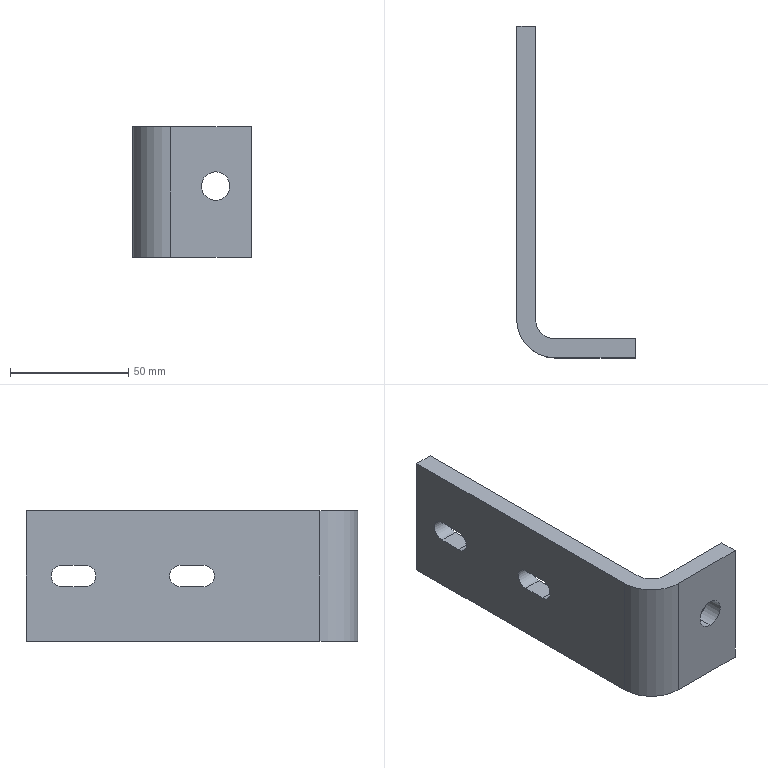Part | STEP file | X77-03031 | 1 solid | 20 faces | box 50 x 140 x 55 mm | volume 74451 mm3 | plane 12 | cylinder 8 | commonest cylinder face diameters 9 x4 12 x2 16 x1 32 x1
STEP:
#1=CARTESIAN_POINT('',(-687.13,-4694.875,24.));
#2=VERTEX_POINT('',#1);
#3=CARTESIAN_POINT('',(-687.13,-4694.875,36.));
#4=VERTEX_POINT('',#3);
#5=CARTESIAN_POINT('',(-687.13,-4694.875,30.));
#6=DIRECTION('',(0.,1.,0.));
#7=DIRECTION('',(0.,0.,1.));
#8=AXIS2_PLACEMENT_3D('',#5,#6,#7);
#9=CIRCLE('',#8,6.);
#10=EDGE_CURVE('',#2,#4,#9,.T.);
#11=ORIENTED_EDGE('',*,*,#10,.F.);
#12=CARTESIAN_POINT('',(-687.13,-4686.875,24.));
#13=VERTEX_POINT('',#12);
#14=CARTESIAN_POINT('',(-687.13,-4746.875,24.));
#15=DIRECTION('',(0.,1.,0.));
#16=VECTOR('',#15,1000.);
#17=LINE('',#14,#16);
#18=EDGE_CURVE('',#2,#13,#17,.T.);
#19=ORIENTED_EDGE('',*,*,#18,.T.);
#20=CARTESIAN_POINT('',(-687.13,-4686.875,36.));
#21=VERTEX_POINT('',#20);
#22=CARTESIAN_POINT('',(-687.13,-4686.875,30.));
#23=DIRECTION('',(0.,1.,0.));
#24=DIRECTION('',(0.,0.,1.));
#25=AXIS2_PLACEMENT_3D('',#22,#23,#24);
#26=CIRCLE('',#25,6.);
#27=EDGE_CURVE('',#13,#21,#26,.T.);
#28=ORIENTED_EDGE('',*,*,#27,.T.);
#29=CARTESIAN_POINT('',(-687.13,-4746.875,36.));
#30=DIRECTION('',(0.,1.,0.));
#31=VECTOR('',#30,1000.);
#32=LINE('',#29,#31);
#33=EDGE_CURVE('',#4,#21,#32,.T.);
#34=ORIENTED_EDGE('',*,*,#33,.F.);
#35=EDGE_LOOP('',(#11,#19,#28,#34));
#36=FACE_OUTER_BOUND('',#35,.T.);
#37=CARTESIAN_POINT('',(-687.13,-4746.875,30.));
#38=DIRECTION('',(0.,1.,0.));
#39=DIRECTION('',(0.,0.,1.));
#40=AXIS2_PLACEMENT_3D('',#37,#38,#39);
#41=CYLINDRICAL_SURFACE('',#40,6.);
#42=ADVANCED_FACE('',(#36),#41,.F.);
#43=CARTESIAN_POINT('',(-714.13,-4554.875,0.));
#44=VERTEX_POINT('',#43);
#45=CARTESIAN_POINT('',(-722.13,-4554.875,0.));
#46=VERTEX_POINT('',#45);
#47=CARTESIAN_POINT('',(-722.13,-4554.875,0.));
#48=DIRECTION('',(-1.,0.,0.));
#49=VECTOR('',#48,1000.);
#50=LINE('',#47,#49);
#51=EDGE_CURVE('',#44,#46,#50,.T.);
#52=ORIENTED_EDGE('',*,*,#51,.T.);
#53=CARTESIAN_POINT('',(-722.13,-4554.875,55.));
#54=VERTEX_POINT('',#53);
#55=CARTESIAN_POINT('',(-722.13,-4554.875,55.));
#56=DIRECTION('',(0.,0.,-1.));
#57=VECTOR('',#56,1000.);
#58=LINE('',#55,#57);
#59=EDGE_CURVE('',#54,#46,#58,.T.);
#60=ORIENTED_EDGE('',*,*,#59,.F.);
#61=CARTESIAN_POINT('',(-714.13,-4554.875,55.));
#62=VERTEX_POINT('',#61);
#63=CARTESIAN_POINT('',(-722.13,-4554.875,55.));
#64=DIRECTION('',(-1.,0.,0.));
#65=VECTOR('',#64,1000.);
#66=LINE('',#63,#65);
#67=EDGE_CURVE('',#62,#54,#66,.T.);
#68=ORIENTED_EDGE('',*,*,#67,.F.);
#69=CARTESIAN_POINT('',(-714.13,-4554.875,55.));
#70=DIRECTION('',(0.,0.,-1.));
#71=VECTOR('',#70,1000.);
#72=LINE('',#69,#71);
#73=EDGE_CURVE('',#62,#44,#72,.T.);
#74=ORIENTED_EDGE('',*,*,#73,.T.);
#75=EDGE_LOOP('',(#52,#60,#68,#74));
#76=FACE_OUTER_BOUND('',#75,.T.);
#77=CARTESIAN_POINT('',(-722.13,-4554.875,55.));
#78=DIRECTION('',(0.,-1.,0.));
#79=DIRECTION('',(0.,0.,-1.));
#80=AXIS2_PLACEMENT_3D('',#77,#78,#79);
#81=PLANE('',#80);
#82=ADVANCED_FACE('',(#76),#81,.F.);
#83=CARTESIAN_POINT('',(-722.13,-4619.875,32.));
#84=VERTEX_POINT('',#83);
#85=CARTESIAN_POINT('',(-722.13,-4629.875,32.));
#86=VERTEX_POINT('',#85);
#87=CARTESIAN_POINT('',(-722.13,-4554.875,32.));
#88=DIRECTION('',(0.,-1.,0.));
#89=VECTOR('',#88,1000.);
#90=LINE('',#87,#89);
#91=EDGE_CURVE('',#84,#86,#90,.T.);
#92=ORIENTED_EDGE('',*,*,#91,.T.);
#93=CARTESIAN_POINT('',(-722.13,-4629.875,23.));
#94=VERTEX_POINT('',#93);
#95=CARTESIAN_POINT('',(-722.13,-4629.875,27.5));
#96=DIRECTION('',(1.,0.,0.));
#97=DIRECTION('',(0.,0.,-1.));
#98=AXIS2_PLACEMENT_3D('',#95,#96,#97);
#99=CIRCLE('',#98,4.5);
#100=EDGE_CURVE('',#86,#94,#99,.T.);
#101=ORIENTED_EDGE('',*,*,#100,.T.);
#102=CARTESIAN_POINT('',(-722.13,-4619.875,23.));
#103=VERTEX_POINT('',#102);
#104=CARTESIAN_POINT('',(-722.13,-4554.875,23.));
#105=DIRECTION('',(0.,1.,0.));
#106=VECTOR('',#105,1000.);
#107=LINE('',#104,#106);
#108=EDGE_CURVE('',#94,#103,#107,.T.);
#109=ORIENTED_EDGE('',*,*,#108,.T.);
#110=CARTESIAN_POINT('',(-722.13,-4619.875,27.5));
#111=DIRECTION('',(1.,0.,0.));
#112=DIRECTION('',(0.,0.,-1.));
#113=AXIS2_PLACEMENT_3D('',#110,#111,#112);
#114=CIRCLE('',#113,4.5);
#115=EDGE_CURVE('',#103,#84,#114,.T.);
#116=ORIENTED_EDGE('',*,*,#115,.T.);
#117=EDGE_LOOP('',(#92,#101,#109,#116));
#118=FACE_BOUND('',#117,.T.);
#119=CARTESIAN_POINT('',(-722.13,-4579.875,23.));
#120=VERTEX_POINT('',#119);
#121=CARTESIAN_POINT('',(-722.13,-4569.875,23.));
#122=VERTEX_POINT('',#121);
#123=CARTESIAN_POINT('',(-722.13,-4554.875,23.));
#124=DIRECTION('',(0.,1.,0.));
#125=VECTOR('',#124,1000.);
#126=LINE('',#123,#125);
#127=EDGE_CURVE('',#120,#122,#126,.T.);
#128=ORIENTED_EDGE('',*,*,#127,.T.);
#129=CARTESIAN_POINT('',(-722.13,-4569.875,32.));
#130=VERTEX_POINT('',#129);
#131=CARTESIAN_POINT('',(-722.13,-4569.875,27.5));
#132=DIRECTION('',(1.,0.,0.));
#133=DIRECTION('',(0.,0.,-1.));
#134=AXIS2_PLACEMENT_3D('',#131,#132,#133);
#135=CIRCLE('',#134,4.5);
#136=EDGE_CURVE('',#122,#130,#135,.T.);
#137=ORIENTED_EDGE('',*,*,#136,.T.);
#138=CARTESIAN_POINT('',(-722.13,-4579.875,32.));
#139=VERTEX_POINT('',#138);
#140=CARTESIAN_POINT('',(-722.13,-4554.875,32.));
#141=DIRECTION('',(0.,-1.,0.));
#142=VECTOR('',#141,1000.);
#143=LINE('',#140,#142);
#144=EDGE_CURVE('',#130,#139,#143,.T.);
#145=ORIENTED_EDGE('',*,*,#144,.T.);
#146=CARTESIAN_POINT('',(-722.13,-4579.875,27.5));
#147=DIRECTION('',(1.,0.,0.));
#148=DIRECTION('',(0.,0.,-1.));
#149=AXIS2_PLACEMENT_3D('',#146,#147,#148);
#150=CIRCLE('',#149,4.5);
#151=EDGE_CURVE('',#139,#120,#150,.T.);
#152=ORIENTED_EDGE('',*,*,#151,.T.);
#153=EDGE_LOOP('',(#128,#137,#145,#152));
#154=FACE_BOUND('',#153,.T.);
#155=CARTESIAN_POINT('',(-722.13,-4678.875,0.));
#156=VERTEX_POINT('',#155);
#157=CARTESIAN_POINT('',(-722.13,-4554.875,0.));
#158=DIRECTION('',(0.,-1.,0.));
#159=VECTOR('',#158,1000.);
#160=LINE('',#157,#159);
#161=EDGE_CURVE('',#46,#156,#160,.T.);
#162=ORIENTED_EDGE('',*,*,#161,.T.);
#163=CARTESIAN_POINT('',(-722.13,-4678.875,55.));
#164=VERTEX_POINT('',#163);
#165=CARTESIAN_POINT('',(-722.13,-4678.875,55.));
#166=DIRECTION('',(0.,0.,1.));
#167=VECTOR('',#166,1000.);
#168=LINE('',#165,#167);
#169=EDGE_CURVE('',#156,#164,#168,.T.);
#170=ORIENTED_EDGE('',*,*,#169,.T.);
#171=CARTESIAN_POINT('',(-722.13,-4554.875,55.));
#172=DIRECTION('',(0.,-1.,0.));
#173=VECTOR('',#172,1000.);
#174=LINE('',#171,#173);
#175=EDGE_CURVE('',#54,#164,#174,.T.);
#176=ORIENTED_EDGE('',*,*,#175,.F.);
#177=ORIENTED_EDGE('',*,*,#59,.T.);
#178=EDGE_LOOP('',(#162,#170,#176,#177));
#179=FACE_OUTER_BOUND('',#178,.T.);
#180=CARTESIAN_POINT('',(-722.13,-4554.875,55.));
#181=DIRECTION('',(1.,0.,0.));
#182=DIRECTION('',(0.,0.,-1.));
#183=AXIS2_PLACEMENT_3D('',#180,#181,#182);
#184=PLANE('',#183);
#185=ADVANCED_FACE('',(#118,#154,#179),#184,.F.);
#186=CARTESIAN_POINT('',(-687.13,-4694.875,30.));
#187=DIRECTION('',(0.,1.,0.));
#188=DIRECTION('',(0.,0.,1.));
#189=AXIS2_PLACEMENT_3D('',#186,#187,#188);
#190=CIRCLE('',#189,6.);
#191=EDGE_CURVE('',#4,#2,#190,.T.);
#192=ORIENTED_EDGE('',*,*,#191,.T.);
#193=ORIENTED_EDGE('',*,*,#10,.T.);
#194=EDGE_LOOP('',(#192,#193));
#195=FACE_BOUND('',#194,.T.);
#196=CARTESIAN_POINT('',(-706.13,-4694.875,55.));
#197=VERTEX_POINT('',#196);
#198=CARTESIAN_POINT('',(-672.13,-4694.875,55.));
#199=VERTEX_POINT('',#198);
#200=CARTESIAN_POINT('',(-672.13,-4694.875,55.));
#201=DIRECTION('',(1.,0.,0.));
#202=VECTOR('',#201,1000.);
#203=LINE('',#200,#202);
#204=EDGE_CURVE('',#197,#199,#203,.T.);
#205=ORIENTED_EDGE('',*,*,#204,.F.);
#206=CARTESIAN_POINT('',(-706.13,-4694.875,0.));
#207=VERTEX_POINT('',#206);
#208=CARTESIAN_POINT('',(-706.13,-4694.875,55.));
#209=DIRECTION('',(0.,0.,-1.));
#210=VECTOR('',#209,1000.);
#211=LINE('',#208,#210);
#212=EDGE_CURVE('',#197,#207,#211,.T.);
#213=ORIENTED_EDGE('',*,*,#212,.T.);
#214=CARTESIAN_POINT('',(-672.13,-4694.875,0.));
#215=VERTEX_POINT('',#214);
#216=CARTESIAN_POINT('',(-672.13,-4694.875,0.));
#217=DIRECTION('',(1.,0.,0.));
#218=VECTOR('',#217,1000.);
#219=LINE('',#216,#218);
#220=EDGE_CURVE('',#207,#215,#219,.T.);
#221=ORIENTED_EDGE('',*,*,#220,.T.);
#222=CARTESIAN_POINT('',(-672.13,-4694.875,55.));
#223=DIRECTION('',(0.,0.,-1.));
#224=VECTOR('',#223,1000.);
#225=LINE('',#222,#224);
#226=EDGE_CURVE('',#199,#215,#225,.T.);
#227=ORIENTED_EDGE('',*,*,#226,.F.);
#228=EDGE_LOOP('',(#205,#213,#221,#227));
#229=FACE_OUTER_BOUND('',#228,.T.);
#230=CARTESIAN_POINT('',(-672.13,-4694.875,55.));
#231=DIRECTION('',(0.,1.,0.));
#232=DIRECTION('',(0.,0.,1.));
#233=AXIS2_PLACEMENT_3D('',#230,#231,#232);
#234=PLANE('',#233);
#235=ADVANCED_FACE('',(#195,#229),#234,.F.);
#236=CARTESIAN_POINT('',(-672.13,-4686.875,0.));
#237=VERTEX_POINT('',#236);
#238=CARTESIAN_POINT('',(-672.13,-4686.875,0.));
#239=DIRECTION('',(0.,1.,0.));
#240=VECTOR('',#239,1000.);
#241=LINE('',#238,#240);
#242=EDGE_CURVE('',#215,#237,#241,.T.);
#243=ORIENTED_EDGE('',*,*,#242,.T.);
#244=CARTESIAN_POINT('',(-672.13,-4686.875,55.));
#245=VERTEX_POINT('',#244);
#246=CARTESIAN_POINT('',(-672.13,-4686.875,55.));
#247=DIRECTION('',(0.,0.,-1.));
#248=VECTOR('',#247,1000.);
#249=LINE('',#246,#248);
#250=EDGE_CURVE('',#245,#237,#249,.T.);
#251=ORIENTED_EDGE('',*,*,#250,.F.);
#252=CARTESIAN_POINT('',(-672.13,-4686.875,55.));
#253=DIRECTION('',(0.,1.,0.));
#254=VECTOR('',#253,1000.);
#255=LINE('',#252,#254);
#256=EDGE_CURVE('',#199,#245,#255,.T.);
#257=ORIENTED_EDGE('',*,*,#256,.F.);
#258=ORIENTED_EDGE('',*,*,#226,.T.);
#259=EDGE_LOOP('',(#243,#251,#257,#258));
#260=FACE_OUTER_BOUND('',#259,.T.);
#261=CARTESIAN_POINT('',(-672.13,-4686.875,55.));
#262=DIRECTION('',(-1.,0.,0.));
#263=DIRECTION('',(0.,0.,1.));
#264=AXIS2_PLACEMENT_3D('',#261,#262,#263);
#265=PLANE('',#264);
#266=ADVANCED_FACE('',(#260),#265,.F.);
#267=CARTESIAN_POINT('',(-687.13,-4686.875,30.));
#268=DIRECTION('',(0.,1.,0.));
#269=DIRECTION('',(0.,0.,1.));
#270=AXIS2_PLACEMENT_3D('',#267,#268,#269);
#271=CIRCLE('',#270,6.);
#272=EDGE_CURVE('',#21,#13,#271,.T.);
#273=ORIENTED_EDGE('',*,*,#272,.F.);
#274=ORIENTED_EDGE('',*,*,#27,.F.);
#275=EDGE_LOOP('',(#273,#274));
#276=FACE_BOUND('',#275,.T.);
#277=CARTESIAN_POINT('',(-706.13,-4686.875,0.));
#278=VERTEX_POINT('',#277);
#279=CARTESIAN_POINT('',(-714.13,-4686.875,0.));
#280=DIRECTION('',(-1.,0.,0.));
#281=VECTOR('',#280,1000.);
#282=LINE('',#279,#281);
#283=EDGE_CURVE('',#237,#278,#282,.T.);
#284=ORIENTED_EDGE('',*,*,#283,.T.);
#285=CARTESIAN_POINT('',(-706.13,-4686.875,55.));
#286=VERTEX_POINT('',#285);
#287=CARTESIAN_POINT('',(-706.13,-4686.875,55.));
#288=DIRECTION('',(0.,0.,1.));
#289=VECTOR('',#288,1000.);
#290=LINE('',#287,#289);
#291=EDGE_CURVE('',#278,#286,#290,.T.);
#292=ORIENTED_EDGE('',*,*,#291,.T.);
#293=CARTESIAN_POINT('',(-714.13,-4686.875,55.));
#294=DIRECTION('',(-1.,0.,0.));
#295=VECTOR('',#294,1000.);
#296=LINE('',#293,#295);
#297=EDGE_CURVE('',#245,#286,#296,.T.);
#298=ORIENTED_EDGE('',*,*,#297,.F.);
#299=ORIENTED_EDGE('',*,*,#250,.T.);
#300=EDGE_LOOP('',(#284,#292,#298,#299));
#301=FACE_OUTER_BOUND('',#300,.T.);
#302=CARTESIAN_POINT('',(-714.13,-4686.875,55.));
#303=DIRECTION('',(0.,-1.,0.));
#304=DIRECTION('',(0.,0.,-1.));
#305=AXIS2_PLACEMENT_3D('',#302,#303,#304);
#306=PLANE('',#305);
#307=ADVANCED_FACE('',(#276,#301),#306,.F.);
#308=CARTESIAN_POINT('',(-714.13,-4629.875,23.));
#309=VERTEX_POINT('',#308);
#310=CARTESIAN_POINT('',(-714.13,-4619.875,23.));
#311=VERTEX_POINT('',#310);
#312=CARTESIAN_POINT('',(-714.13,-4629.875,23.));
#313=DIRECTION('',(0.,1.,0.));
#314=VECTOR('',#313,1000.);
#315=LINE('',#312,#314);
#316=EDGE_CURVE('',#309,#311,#315,.T.);
#317=ORIENTED_EDGE('',*,*,#316,.F.);
#318=CARTESIAN_POINT('',(-714.13,-4629.875,32.));
#319=VERTEX_POINT('',#318);
#320=CARTESIAN_POINT('',(-714.13,-4629.875,27.5));
#321=DIRECTION('',(1.,0.,0.));
#322=DIRECTION('',(0.,0.,-1.));
#323=AXIS2_PLACEMENT_3D('',#320,#321,#322);
#324=CIRCLE('',#323,4.5);
#325=EDGE_CURVE('',#319,#309,#324,.T.);
#326=ORIENTED_EDGE('',*,*,#325,.F.);
#327=CARTESIAN_POINT('',(-714.13,-4619.875,32.));
#328=VERTEX_POINT('',#327);
#329=CARTESIAN_POINT('',(-714.13,-4629.875,32.));
#330=DIRECTION('',(0.,-1.,0.));
#331=VECTOR('',#330,1000.);
#332=LINE('',#329,#331);
#333=EDGE_CURVE('',#328,#319,#332,.T.);
#334=ORIENTED_EDGE('',*,*,#333,.F.);
#335=CARTESIAN_POINT('',(-714.13,-4619.875,27.5));
#336=DIRECTION('',(1.,0.,0.));
#337=DIRECTION('',(0.,0.,-1.));
#338=AXIS2_PLACEMENT_3D('',#335,#336,#337);
#339=CIRCLE('',#338,4.5);
#340=EDGE_CURVE('',#311,#328,#339,.T.);
#341=ORIENTED_EDGE('',*,*,#340,.F.);
#342=EDGE_LOOP('',(#317,#326,#334,#341));
#343=FACE_BOUND('',#342,.T.);
#344=CARTESIAN_POINT('',(-714.13,-4569.875,32.));
#345=VERTEX_POINT('',#344);
#346=CARTESIAN_POINT('',(-714.13,-4579.875,32.));
#347=VERTEX_POINT('',#346);
#348=CARTESIAN_POINT('',(-714.13,-4569.875,32.));
#349=DIRECTION('',(0.,-1.,0.));
#350=VECTOR('',#349,1000.);
#351=LINE('',#348,#350);
#352=EDGE_CURVE('',#345,#347,#351,.T.);
#353=ORIENTED_EDGE('',*,*,#352,.F.);
#354=CARTESIAN_POINT('',(-714.13,-4569.875,23.));
#355=VERTEX_POINT('',#354);
#356=CARTESIAN_POINT('',(-714.13,-4569.875,27.5));
#357=DIRECTION('',(1.,0.,0.));
#358=DIRECTION('',(0.,0.,-1.));
#359=AXIS2_PLACEMENT_3D('',#356,#357,#358);
#360=CIRCLE('',#359,4.5);
#361=EDGE_CURVE('',#355,#345,#360,.T.);
#362=ORIENTED_EDGE('',*,*,#361,.F.);
#363=CARTESIAN_POINT('',(-714.13,-4579.875,23.));
#364=VERTEX_POINT('',#363);
#365=CARTESIAN_POINT('',(-714.13,-4569.875,23.));
#366=DIRECTION('',(0.,1.,0.));
#367=VECTOR('',#366,1000.);
#368=LINE('',#365,#367);
#369=EDGE_CURVE('',#364,#355,#368,.T.);
#370=ORIENTED_EDGE('',*,*,#369,.F.);
#371=CARTESIAN_POINT('',(-714.13,-4579.875,27.5));
#372=DIRECTION('',(1.,0.,0.));
#373=DIRECTION('',(0.,0.,-1.));
#374=AXIS2_PLACEMENT_3D('',#371,#372,#373);
#375=CIRCLE('',#374,4.5);
#376=EDGE_CURVE('',#347,#364,#375,.T.);
#377=ORIENTED_EDGE('',*,*,#376,.F.);
#378=EDGE_LOOP('',(#353,#362,#370,#377));
#379=FACE_BOUND('',#378,.T.);
#380=CARTESIAN_POINT('',(-714.13,-4678.875,55.));
#381=VERTEX_POINT('',#380);
#382=CARTESIAN_POINT('',(-714.13,-4554.875,55.));
#383=DIRECTION('',(0.,1.,0.));
#384=VECTOR('',#383,1000.);
#385=LINE('',#382,#384);
#386=EDGE_CURVE('',#381,#62,#385,.T.);
#387=ORIENTED_EDGE('',*,*,#386,.F.);
#388=CARTESIAN_POINT('',(-714.13,-4678.875,0.));
#389=VERTEX_POINT('',#388);
#390=CARTESIAN_POINT('',(-714.13,-4678.875,0.));
#391=DIRECTION('',(0.,0.,-1.));
#392=VECTOR('',#391,1000.);
#393=LINE('',#390,#392);
#394=EDGE_CURVE('',#381,#389,#393,.T.);
#395=ORIENTED_EDGE('',*,*,#394,.T.);
#396=CARTESIAN_POINT('',(-714.13,-4554.875,0.));
#397=DIRECTION('',(0.,1.,0.));
#398=VECTOR('',#397,1000.);
#399=LINE('',#396,#398);
#400=EDGE_CURVE('',#389,#44,#399,.T.);
#401=ORIENTED_EDGE('',*,*,#400,.T.);
#402=ORIENTED_EDGE('',*,*,#73,.F.);
#403=EDGE_LOOP('',(#387,#395,#401,#402));
#404=FACE_OUTER_BOUND('',#403,.T.);
#405=CARTESIAN_POINT('',(-714.13,-4554.875,55.));
#406=DIRECTION('',(-1.,0.,0.));
#407=DIRECTION('',(0.,0.,1.));
#408=AXIS2_PLACEMENT_3D('',#405,#406,#407);
#409=PLANE('',#408);
#410=ADVANCED_FACE('',(#343,#379,#404),#409,.F.);
#411=ORIENTED_EDGE('',*,*,#175,.T.);
#412=CARTESIAN_POINT('',(-706.13,-4678.875,55.));
#413=DIRECTION('',(0.,0.,1.));
#414=DIRECTION('',(-1.,0.,0.));
#415=AXIS2_PLACEMENT_3D('',#412,#413,#414);
#416=CIRCLE('',#415,16.);
#417=EDGE_CURVE('',#164,#197,#416,.T.);
#418=ORIENTED_EDGE('',*,*,#417,.T.);
#419=ORIENTED_EDGE('',*,*,#204,.T.);
#420=ORIENTED_EDGE('',*,*,#256,.T.);
#421=ORIENTED_EDGE('',*,*,#297,.T.);
#422=CARTESIAN_POINT('',(-706.13,-4678.875,55.));
#423=DIRECTION('',(0.,0.,-1.));
#424=DIRECTION('',(-1.,0.,0.));
#425=AXIS2_PLACEMENT_3D('',#422,#423,#424);
#426=CIRCLE('',#425,8.);
#427=EDGE_CURVE('',#286,#381,#426,.T.);
#428=ORIENTED_EDGE('',*,*,#427,.T.);
#429=ORIENTED_EDGE('',*,*,#386,.T.);
#430=ORIENTED_EDGE('',*,*,#67,.T.);
#431=EDGE_LOOP('',(#411,#418,#419,#420,#421,#428,#429,#430));
#432=FACE_OUTER_BOUND('',#431,.T.);
#433=CARTESIAN_POINT('',(-714.13,-4554.875,55.));
#434=DIRECTION('',(0.,0.,-1.));
#435=DIRECTION('',(-1.,0.,0.));
#436=AXIS2_PLACEMENT_3D('',#433,#434,#435);
#437=PLANE('',#436);
#438=ADVANCED_FACE('',(#432),#437,.F.);
#439=ORIENTED_EDGE('',*,*,#220,.F.);
#440=CARTESIAN_POINT('',(-706.13,-4678.875,0.));
#441=DIRECTION('',(0.,0.,-1.));
#442=DIRECTION('',(-1.,0.,0.));
#443=AXIS2_PLACEMENT_3D('',#440,#441,#442);
#444=CIRCLE('',#443,16.);
#445=EDGE_CURVE('',#207,#156,#444,.T.);
#446=ORIENTED_EDGE('',*,*,#445,.T.);
#447=ORIENTED_EDGE('',*,*,#161,.F.);
#448=ORIENTED_EDGE('',*,*,#51,.F.);
#449=ORIENTED_EDGE('',*,*,#400,.F.);
#450=CARTESIAN_POINT('',(-706.13,-4678.875,0.));
#451=DIRECTION('',(0.,0.,1.));
#452=DIRECTION('',(-1.,0.,0.));
#453=AXIS2_PLACEMENT_3D('',#450,#451,#452);
#454=CIRCLE('',#453,8.);
#455=EDGE_CURVE('',#389,#278,#454,.T.);
#456=ORIENTED_EDGE('',*,*,#455,.T.);
#457=ORIENTED_EDGE('',*,*,#283,.F.);
#458=ORIENTED_EDGE('',*,*,#242,.F.);
#459=EDGE_LOOP('',(#439,#446,#447,#448,#449,#456,#457,#458));
#460=FACE_OUTER_BOUND('',#459,.T.);
#461=CARTESIAN_POINT('',(-714.13,-4554.875,0.));
#462=DIRECTION('',(0.,0.,-1.));
#463=DIRECTION('',(-1.,0.,0.));
#464=AXIS2_PLACEMENT_3D('',#461,#462,#463);
#465=PLANE('',#464);
#466=ADVANCED_FACE('',(#460),#465,.T.);
#467=ORIENTED_EDGE('',*,*,#18,.F.);
#468=ORIENTED_EDGE('',*,*,#191,.F.);
#469=ORIENTED_EDGE('',*,*,#33,.T.);
#470=ORIENTED_EDGE('',*,*,#272,.T.);
#471=EDGE_LOOP('',(#467,#468,#469,#470));
#472=FACE_OUTER_BOUND('',#471,.T.);
#473=CARTESIAN_POINT('',(-687.13,-4746.875,30.));
#474=DIRECTION('',(0.,1.,0.));
#475=DIRECTION('',(0.,0.,1.));
#476=AXIS2_PLACEMENT_3D('',#473,#474,#475);
#477=CYLINDRICAL_SURFACE('',#476,6.);
#478=ADVANCED_FACE('',(#472),#477,.F.);
#479=ORIENTED_EDGE('',*,*,#427,.F.);
#480=ORIENTED_EDGE('',*,*,#291,.F.);
#481=ORIENTED_EDGE('',*,*,#455,.F.);
#482=ORIENTED_EDGE('',*,*,#394,.F.);
#483=EDGE_LOOP('',(#479,#480,#481,#482));
#484=FACE_OUTER_BOUND('',#483,.T.);
#485=CARTESIAN_POINT('',(-706.13,-4678.875,55.));
#486=DIRECTION('',(0.,0.,1.));
#487=DIRECTION('',(1.,0.,0.));
#488=AXIS2_PLACEMENT_3D('',#485,#486,#487);
#489=CYLINDRICAL_SURFACE('',#488,8.);
#490=ADVANCED_FACE('',(#484),#489,.F.);
#491=ORIENTED_EDGE('',*,*,#417,.F.);
#492=ORIENTED_EDGE('',*,*,#169,.F.);
#493=ORIENTED_EDGE('',*,*,#445,.F.);
#494=ORIENTED_EDGE('',*,*,#212,.F.);
#495=EDGE_LOOP('',(#491,#492,#493,#494));
#496=FACE_OUTER_BOUND('',#495,.T.);
#497=CARTESIAN_POINT('',(-706.13,-4678.875,55.));
#498=DIRECTION('',(0.,0.,-1.));
#499=DIRECTION('',(-1.,0.,0.));
#500=AXIS2_PLACEMENT_3D('',#497,#498,#499);
#501=CYLINDRICAL_SURFACE('',#500,16.);
#502=ADVANCED_FACE('',(#496),#501,.T.);
#503=CARTESIAN_POINT('',(-774.13,-4569.875,23.));
#504=DIRECTION('',(1.,0.,0.));
#505=VECTOR('',#504,1000.);
#506=LINE('',#503,#505);
#507=EDGE_CURVE('',#122,#355,#506,.T.);
#508=ORIENTED_EDGE('',*,*,#507,.T.);
#509=ORIENTED_EDGE('',*,*,#361,.T.);
#510=CARTESIAN_POINT('',(-774.13,-4569.875,32.));
#511=DIRECTION('',(1.,0.,0.));
#512=VECTOR('',#511,1000.);
#513=LINE('',#510,#512);
#514=EDGE_CURVE('',#130,#345,#513,.T.);
#515=ORIENTED_EDGE('',*,*,#514,.F.);
#516=ORIENTED_EDGE('',*,*,#136,.F.);
#517=EDGE_LOOP('',(#508,#509,#515,#516));
#518=FACE_OUTER_BOUND('',#517,.T.);
#519=CARTESIAN_POINT('',(-774.13,-4569.875,27.5));
#520=DIRECTION('',(1.,0.,0.));
#521=DIRECTION('',(0.,0.,-1.));
#522=AXIS2_PLACEMENT_3D('',#519,#520,#521);
#523=CYLINDRICAL_SURFACE('',#522,4.5);
#524=ADVANCED_FACE('',(#518),#523,.F.);
#525=CARTESIAN_POINT('',(-774.13,-4579.875,23.));
#526=DIRECTION('',(1.,0.,0.));
#527=VECTOR('',#526,1000.);
#528=LINE('',#525,#527);
#529=EDGE_CURVE('',#120,#364,#528,.T.);
#530=ORIENTED_EDGE('',*,*,#529,.T.);
#531=ORIENTED_EDGE('',*,*,#369,.T.);
#532=ORIENTED_EDGE('',*,*,#507,.F.);
#533=ORIENTED_EDGE('',*,*,#127,.F.);
#534=EDGE_LOOP('',(#530,#531,#532,#533));
#535=FACE_OUTER_BOUND('',#534,.T.);
#536=CARTESIAN_POINT('',(-774.13,-4569.875,23.));
#537=DIRECTION('',(0.,0.,-1.));
#538=DIRECTION('',(0.,1.,0.));
#539=AXIS2_PLACEMENT_3D('',#536,#537,#538);
#540=PLANE('',#539);
#541=ADVANCED_FACE('',(#535),#540,.F.);
#542=CARTESIAN_POINT('',(-774.13,-4579.875,32.));
#543=DIRECTION('',(1.,0.,0.));
#544=VECTOR('',#543,1000.);
#545=LINE('',#542,#544);
#546=EDGE_CURVE('',#139,#347,#545,.T.);
#547=ORIENTED_EDGE('',*,*,#546,.T.);
#548=ORIENTED_EDGE('',*,*,#376,.T.);
#549=ORIENTED_EDGE('',*,*,#529,.F.);
#550=ORIENTED_EDGE('',*,*,#151,.F.);
#551=EDGE_LOOP('',(#547,#548,#549,#550));
#552=FACE_OUTER_BOUND('',#551,.T.);
#553=CARTESIAN_POINT('',(-774.13,-4579.875,27.5));
#554=DIRECTION('',(1.,0.,0.));
#555=DIRECTION('',(0.,0.,-1.));
#556=AXIS2_PLACEMENT_3D('',#553,#554,#555);
#557=CYLINDRICAL_SURFACE('',#556,4.5);
#558=ADVANCED_FACE('',(#552),#557,.F.);
#559=ORIENTED_EDGE('',*,*,#514,.T.);
#560=ORIENTED_EDGE('',*,*,#352,.T.);
#561=ORIENTED_EDGE('',*,*,#546,.F.);
#562=ORIENTED_EDGE('',*,*,#144,.F.);
#563=EDGE_LOOP('',(#559,#560,#561,#562));
#564=FACE_OUTER_BOUND('',#563,.T.);
#565=CARTESIAN_POINT('',(-774.13,-4569.875,32.));
#566=DIRECTION('',(0.,0.,1.));
#567=DIRECTION('',(1.,0.,0.));
#568=AXIS2_PLACEMENT_3D('',#565,#566,#567);
#569=PLANE('',#568);
#570=ADVANCED_FACE('',(#564),#569,.F.);
#571=CARTESIAN_POINT('',(-774.13,-4629.875,32.));
#572=DIRECTION('',(1.,0.,0.));
#573=VECTOR('',#572,1000.);
#574=LINE('',#571,#573);
#575=EDGE_CURVE('',#86,#319,#574,.T.);
#576=ORIENTED_EDGE('',*,*,#575,.T.);
#577=ORIENTED_EDGE('',*,*,#325,.T.);
#578=CARTESIAN_POINT('',(-774.13,-4629.875,23.));
#579=DIRECTION('',(1.,0.,0.));
#580=VECTOR('',#579,1000.);
#581=LINE('',#578,#580);
#582=EDGE_CURVE('',#94,#309,#581,.T.);
#583=ORIENTED_EDGE('',*,*,#582,.F.);
#584=ORIENTED_EDGE('',*,*,#100,.F.);
#585=EDGE_LOOP('',(#576,#577,#583,#584));
#586=FACE_OUTER_BOUND('',#585,.T.);
#587=CARTESIAN_POINT('',(-774.13,-4629.875,27.5));
#588=DIRECTION('',(1.,0.,0.));
#589=DIRECTION('',(0.,0.,-1.));
#590=AXIS2_PLACEMENT_3D('',#587,#588,#589);
#591=CYLINDRICAL_SURFACE('',#590,4.5);
#592=ADVANCED_FACE('',(#586),#591,.F.);
#593=CARTESIAN_POINT('',(-774.13,-4619.875,32.));
#594=DIRECTION('',(1.,0.,0.));
#595=VECTOR('',#594,1000.);
#596=LINE('',#593,#595);
#597=EDGE_CURVE('',#84,#328,#596,.T.);
#598=ORIENTED_EDGE('',*,*,#597,.T.);
#599=ORIENTED_EDGE('',*,*,#333,.T.);
#600=ORIENTED_EDGE('',*,*,#575,.F.);
#601=ORIENTED_EDGE('',*,*,#91,.F.);
#602=EDGE_LOOP('',(#598,#599,#600,#601));
#603=FACE_OUTER_BOUND('',#602,.T.);
#604=CARTESIAN_POINT('',(-774.13,-4629.875,32.));
#605=DIRECTION('',(0.,0.,1.));
#606=DIRECTION('',(1.,0.,0.));
#607=AXIS2_PLACEMENT_3D('',#604,#605,#606);
#608=PLANE('',#607);
#609=ADVANCED_FACE('',(#603),#608,.F.);
#610=CARTESIAN_POINT('',(-774.13,-4619.875,23.));
#611=DIRECTION('',(1.,0.,0.));
#612=VECTOR('',#611,1000.);
#613=LINE('',#610,#612);
#614=EDGE_CURVE('',#103,#311,#613,.T.);
#615=ORIENTED_EDGE('',*,*,#614,.T.);
#616=ORIENTED_EDGE('',*,*,#340,.T.);
#617=ORIENTED_EDGE('',*,*,#597,.F.);
#618=ORIENTED_EDGE('',*,*,#115,.F.);
#619=EDGE_LOOP('',(#615,#616,#617,#618));
#620=FACE_OUTER_BOUND('',#619,.T.);
#621=CARTESIAN_POINT('',(-774.13,-4619.875,27.5));
#622=DIRECTION('',(1.,0.,0.));
#623=DIRECTION('',(0.,0.,-1.));
#624=AXIS2_PLACEMENT_3D('',#621,#622,#623);
#625=CYLINDRICAL_SURFACE('',#624,4.5);
#626=ADVANCED_FACE('',(#620),#625,.F.);
#627=ORIENTED_EDGE('',*,*,#582,.T.);
#628=ORIENTED_EDGE('',*,*,#316,.T.);
#629=ORIENTED_EDGE('',*,*,#614,.F.);
#630=ORIENTED_EDGE('',*,*,#108,.F.);
#631=EDGE_LOOP('',(#627,#628,#629,#630));
#632=FACE_OUTER_BOUND('',#631,.T.);
#633=CARTESIAN_POINT('',(-774.13,-4629.875,23.));
#634=DIRECTION('',(0.,0.,-1.));
#635=DIRECTION('',(0.,1.,0.));
#636=AXIS2_PLACEMENT_3D('',#633,#634,#635);
#637=PLANE('',#636);
#638=ADVANCED_FACE('',(#632),#637,.F.);
#639=CLOSED_SHELL('',(#42,#82,#185,#235,#266,#307,#410,#438,#466,#478,#490,#502,#524,#541,#558,#570,#592,#609,#626,#638));
#640=MANIFOLD_SOLID_BREP('',#639);
#641=CARTESIAN_POINT('',(0.,0.,0.));
#642=DIRECTION('',(0.,0.,1.));
#643=DIRECTION('',(1.,0.,0.));
#644=AXIS2_PLACEMENT_3D('',#641,#642,#643);
#645=(LENGTH_UNIT()NAMED_UNIT(*)SI_UNIT(.MILLI.,.METRE.));
#646=UNCERTAINTY_MEASURE_WITH_UNIT(LENGTH_MEASURE(0.00001),#645,'','');
#647=(NAMED_UNIT(*)PLANE_ANGLE_UNIT()SI_UNIT($,.RADIAN.));
#648=(NAMED_UNIT(*)SI_UNIT($,.STERADIAN.)SOLID_ANGLE_UNIT());
#649=(GEOMETRIC_REPRESENTATION_CONTEXT(3)GLOBAL_UNCERTAINTY_ASSIGNED_CONTEXT((#646))GLOBAL_UNIT_ASSIGNED_CONTEXT((#645,#647,#648))REPRESENTATION_CONTEXT('',''));
#650=ADVANCED_BREP_SHAPE_REPRESENTATION('',(#640,#644),#649);